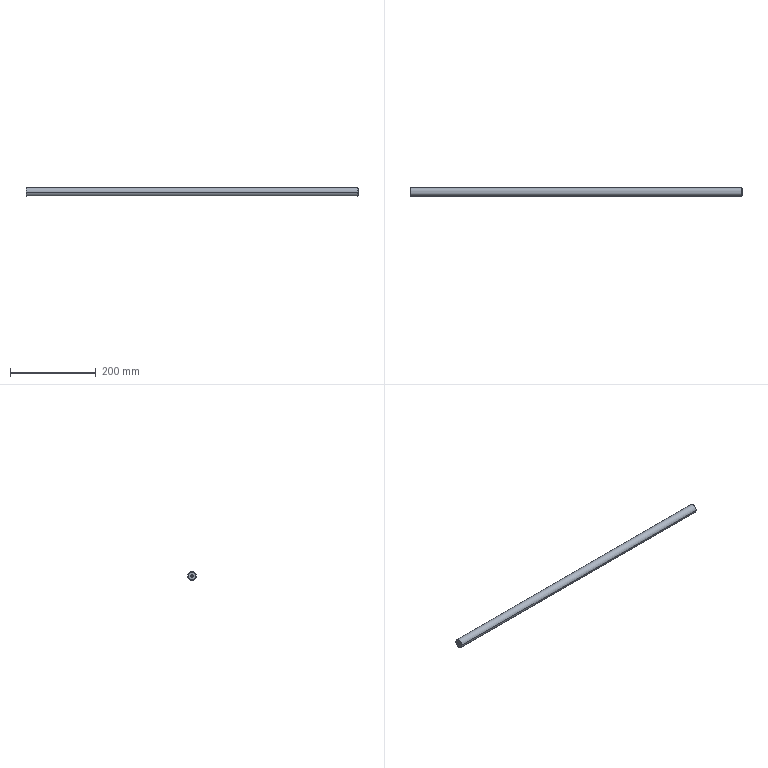Part | STEP file | 03-23 Lead screw guide shaft | 1 solid | 16 faces | box 775 x 20 x 20 mm | volume 242804 mm3 | cone 8 | cylinder 6 | plane 2 | commonest cylinder face diameters 5 x4 20 x2